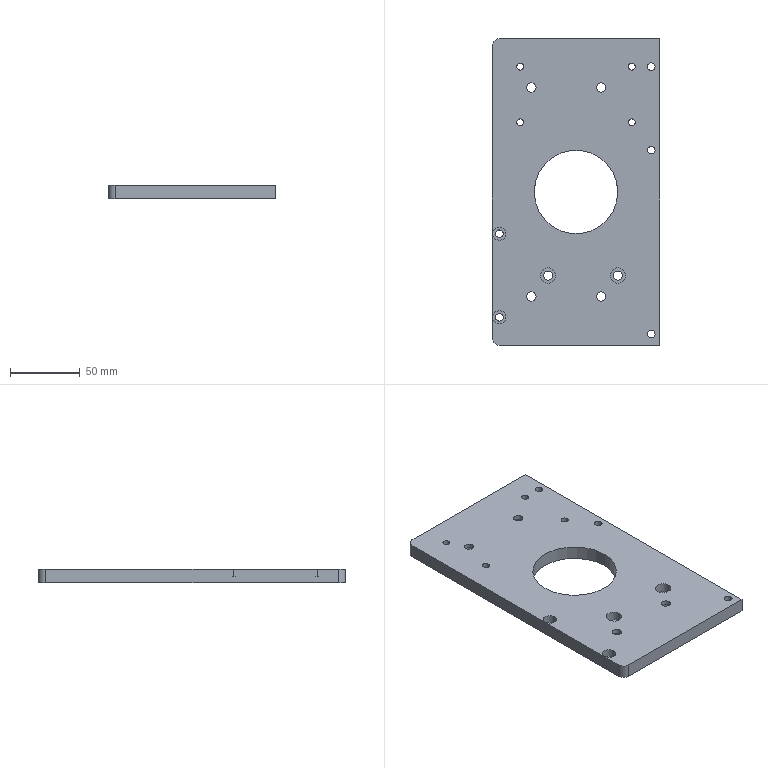Part | SolidWorks | features HoleWzd 5, Extrusion 1, Fillet 1, ICE 1 | 1 solid | 73 faces | box 120 x 220 x 10 mm | volume 227637 mm3 | cylinder 56 | plane 17 | commonest cylinder face diameters 6.6 x12 11 x12 5.5 x10 5 x8 10 x8 9.5 x4